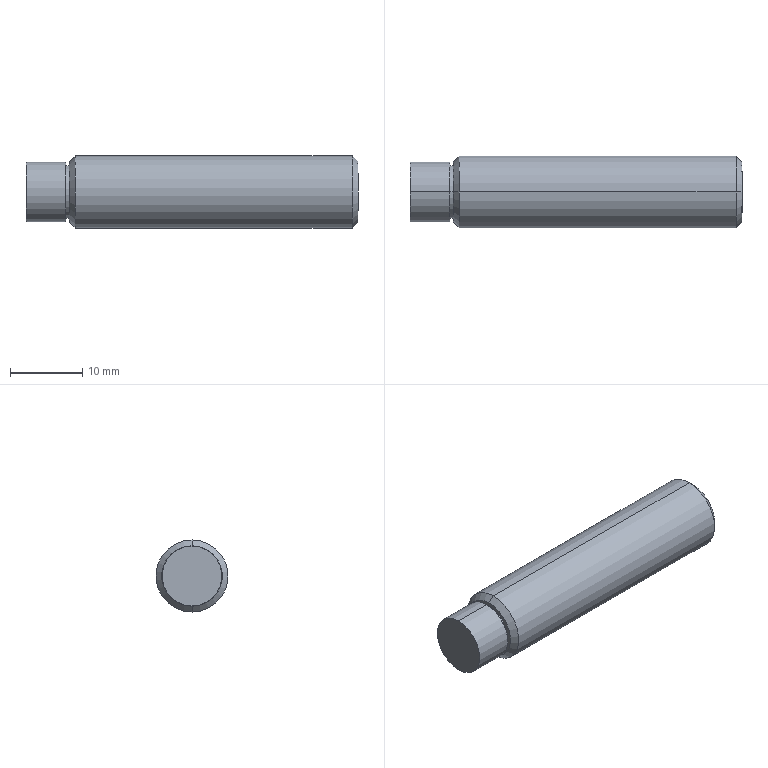Part | STEP file | 0217_Z_PUSS10-40-1 | 1 solid | 28 faces | box 46 x 10 x 10 mm | volume 3323 mm3 | plane 16 | cylinder 6 | cone 6 | commonest cylinder face diameters 7.3 x2 8.3 x2 10 x2